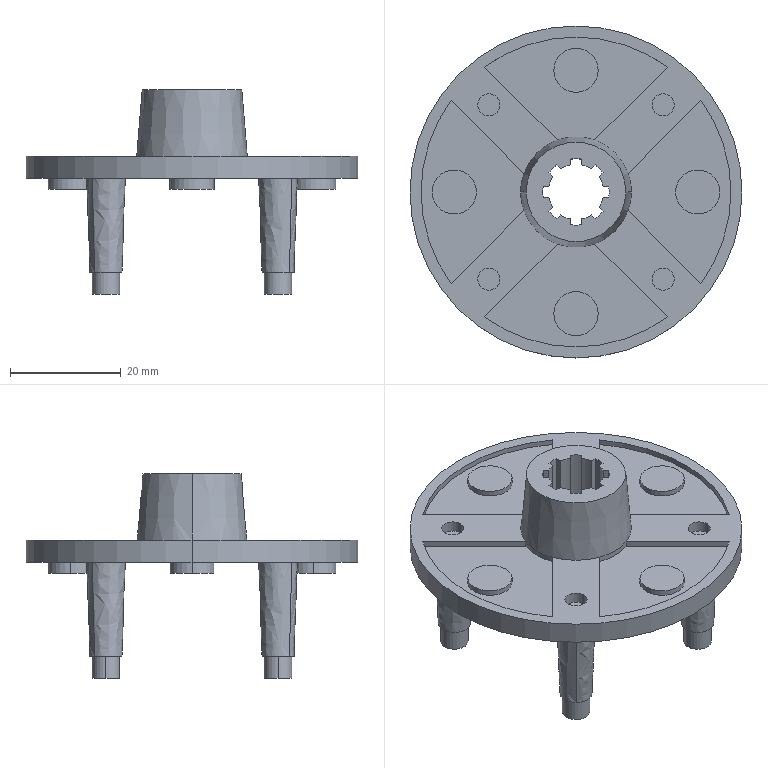Part | SolidWorks | features ICE 8, CirPattern 5, Blend 1, Extrusion 1, Revolution 1 | 1 solid | 146 faces | box 60 x 60 x 37 mm | volume 14280 mm3 | cylinder 77 | plane 59 | spline 8 | cone 2 | commonest cylinder face diameters 5 x16 8 x16 12 x9 3 x8 4 x8 10 x8